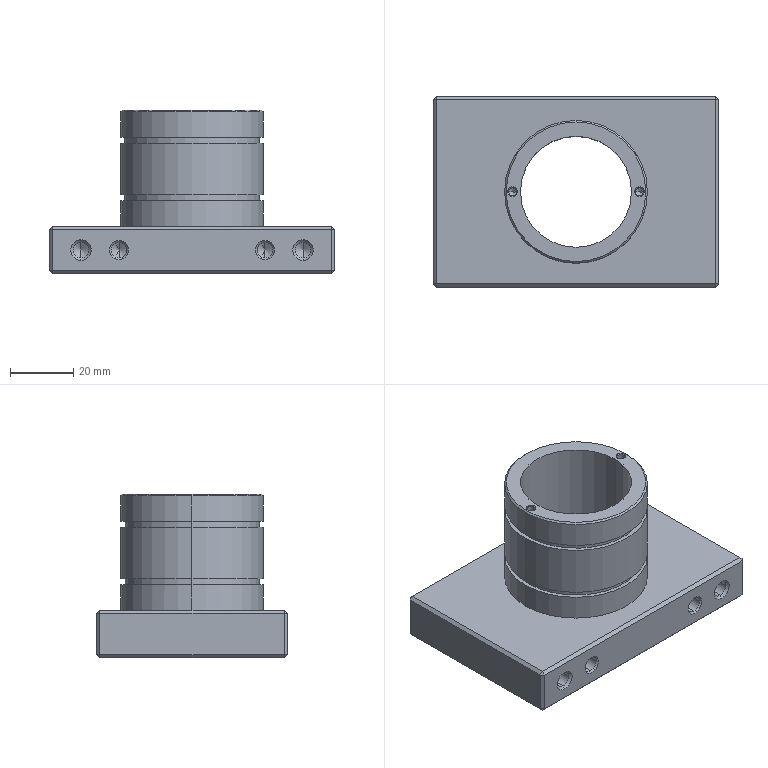Part | SolidWorks | features Chamfer 6, HoleWzd 5, ICE 5, Cut 2, Extrusion 1, MoveFace 1 | 2 solids | 122 faces | box 90 x 60 x 51.6 mm | volume 84781 mm3 | cone 52 | cylinder 38 | plane 32 | commonest cylinder face diameters 5 x20 45 x8 2.5 x4 42.5 x4 35 x2